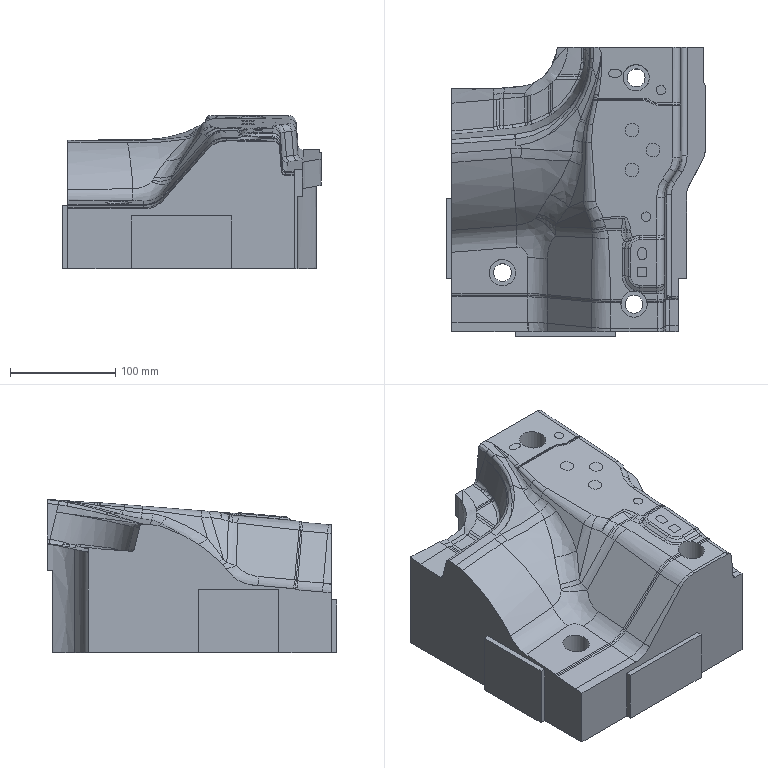Part | NX | features solid 2 | 1 solid | 266 faces | box 245.737 x 275 x 145.496 mm | volume 6126367 mm3 | spline 139 | cylinder 75 | plane 46 | torus 3 | sphere 3 | commonest cylinder face diameters 10 x17 6 x14 14 x7 20 x5 10.001 x3 17 x3